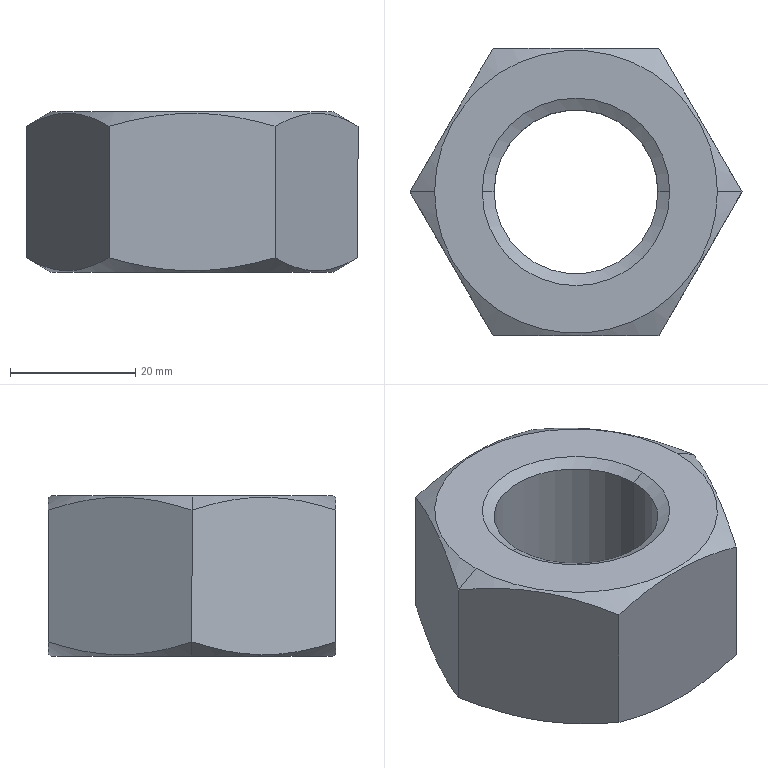Part | SolidWorks | features RevCut 2, Chamfer 1, Extrusion 1, LPattern 1 | 1 solid | 18 faces | box 53.116 x 46 x 25.6 mm | volume 32625 mm3 | cone 8 | plane 8 | cylinder 2 | commonest cylinder face diameters 26.211 x2
STEP:
#1=CARTESIAN_POINT('',(-13.106,0.,-1.094));
#2=VERTEX_POINT('',#1);
#3=CARTESIAN_POINT('',(13.106,0.,-1.094));
#4=VERTEX_POINT('',#3);
#5=CARTESIAN_POINT('',(0.,0.,-1.094));
#6=DIRECTION('',(0.,0.,1.));
#7=DIRECTION('',(1.,0.,0.));
#8=AXIS2_PLACEMENT_3D('',#5,#6,#7);
#9=CIRCLE('',#8,13.106);
#10=EDGE_CURVE('',#2,#4,#9,.T.);
#11=ORIENTED_EDGE('',*,*,#10,.F.);
#12=CARTESIAN_POINT('',(-15.,0.,0.));
#13=VERTEX_POINT('',#12);
#14=CARTESIAN_POINT('',(-13.106,0.,-1.094));
#15=DIRECTION('',(-0.866,0.,0.5));
#16=VECTOR('',#15,1000.);
#17=LINE('',#14,#16);
#18=EDGE_CURVE('',#2,#13,#17,.T.);
#19=ORIENTED_EDGE('',*,*,#18,.T.);
#20=CARTESIAN_POINT('',(15.,0.,0.));
#21=VERTEX_POINT('',#20);
#22=CARTESIAN_POINT('',(0.,0.,0.));
#23=DIRECTION('',(0.,0.,-1.));
#24=DIRECTION('',(1.,0.,0.));
#25=AXIS2_PLACEMENT_3D('',#22,#23,#24);
#26=CIRCLE('',#25,15.);
#27=EDGE_CURVE('',#21,#13,#26,.T.);
#28=ORIENTED_EDGE('',*,*,#27,.F.);
#29=CARTESIAN_POINT('',(13.106,0.,-1.094));
#30=DIRECTION('',(0.866,0.,0.5));
#31=VECTOR('',#30,1000.);
#32=LINE('',#29,#31);
#33=EDGE_CURVE('',#4,#21,#32,.T.);
#34=ORIENTED_EDGE('',*,*,#33,.F.);
#35=EDGE_LOOP('',(#11,#19,#28,#34));
#36=FACE_OUTER_BOUND('',#35,.T.);
#37=CARTESIAN_POINT('',(0.,0.,-1.094));
#38=DIRECTION('',(0.,0.,1.));
#39=DIRECTION('',(1.,0.,0.));
#40=AXIS2_PLACEMENT_3D('',#37,#38,#39);
#41=CONICAL_SURFACE('',#40,13.106,1.047);
#42=ADVANCED_FACE('',(#36),#41,.F.);
#43=CARTESIAN_POINT('',(13.106,0.,-23.705));
#44=VERTEX_POINT('',#43);
#45=CARTESIAN_POINT('',(-13.106,0.,-23.705));
#46=VERTEX_POINT('',#45);
#47=CARTESIAN_POINT('',(0.,0.,-23.705));
#48=DIRECTION('',(0.,0.,-1.));
#49=DIRECTION('',(1.,0.,0.));
#50=AXIS2_PLACEMENT_3D('',#47,#48,#49);
#51=CIRCLE('',#50,13.106);
#52=EDGE_CURVE('',#44,#46,#51,.T.);
#53=ORIENTED_EDGE('',*,*,#52,.F.);
#54=CARTESIAN_POINT('',(14.199,0.,-25.6));
#55=VERTEX_POINT('',#54);
#56=CARTESIAN_POINT('',(14.199,0.,-25.6));
#57=DIRECTION('',(0.5,0.,-0.866));
#58=VECTOR('',#57,1000.);
#59=LINE('',#56,#58);
#60=EDGE_CURVE('',#44,#55,#59,.T.);
#61=ORIENTED_EDGE('',*,*,#60,.T.);
#62=CARTESIAN_POINT('',(-14.199,0.,-25.6));
#63=VERTEX_POINT('',#62);
#64=CARTESIAN_POINT('',(0.,0.,-25.6));
#65=DIRECTION('',(0.,0.,1.));
#66=DIRECTION('',(1.,0.,0.));
#67=AXIS2_PLACEMENT_3D('',#64,#65,#66);
#68=CIRCLE('',#67,14.199);
#69=EDGE_CURVE('',#63,#55,#68,.T.);
#70=ORIENTED_EDGE('',*,*,#69,.F.);
#71=CARTESIAN_POINT('',(-14.199,0.,-25.6));
#72=DIRECTION('',(-0.5,0.,-0.866));
#73=VECTOR('',#72,1000.);
#74=LINE('',#71,#73);
#75=EDGE_CURVE('',#46,#63,#74,.T.);
#76=ORIENTED_EDGE('',*,*,#75,.F.);
#77=EDGE_LOOP('',(#53,#61,#70,#76));
#78=FACE_OUTER_BOUND('',#77,.T.);
#79=CARTESIAN_POINT('',(0.,0.,-25.6));
#80=DIRECTION('',(0.,0.,-1.));
#81=DIRECTION('',(-1.,0.,0.));
#82=AXIS2_PLACEMENT_3D('',#79,#80,#81);
#83=CONICAL_SURFACE('',#82,14.199,0.5236);
#84=ADVANCED_FACE('',(#78),#83,.F.);
#85=CARTESIAN_POINT('',(-22.625,0.,0.));
#86=VERTEX_POINT('',#85);
#87=CARTESIAN_POINT('',(22.625,0.,0.));
#88=VERTEX_POINT('',#87);
#89=CARTESIAN_POINT('',(0.,0.,0.));
#90=DIRECTION('',(0.,0.,-1.));
#91=DIRECTION('',(-1.,0.,0.));
#92=AXIS2_PLACEMENT_3D('',#89,#90,#91);
#93=CIRCLE('',#92,22.625);
#94=EDGE_CURVE('',#86,#88,#93,.T.);
#95=ORIENTED_EDGE('',*,*,#94,.T.);
#96=CARTESIAN_POINT('',(26.558,0.,-2.271));
#97=VERTEX_POINT('',#96);
#98=CARTESIAN_POINT('',(22.625,0.,0.));
#99=DIRECTION('',(0.866,0.,-0.5));
#100=VECTOR('',#99,1000.);
#101=LINE('',#98,#100);
#102=EDGE_CURVE('',#88,#97,#101,.T.);
#103=ORIENTED_EDGE('',*,*,#102,.T.);
#104=CARTESIAN_POINT('',(13.279,23.,-2.271));
#105=VERTEX_POINT('',#104);
#106=CARTESIAN_POINT('',(26.558,0.,-2.271));
#107=CARTESIAN_POINT('',(25.474,1.878,-1.645));
#108=CARTESIAN_POINT('',(24.382,3.769,-1.129));
#109=CARTESIAN_POINT('',(22.175,7.591,-0.4144));
#110=CARTESIAN_POINT('',(21.06,9.523,-0.218));
#111=CARTESIAN_POINT('',(19.649,11.967,-0.2162));
#112=CARTESIAN_POINT('',(19.365,12.458,-0.2279));
#113=CARTESIAN_POINT('',(18.801,13.436,-0.2751));
#114=CARTESIAN_POINT('',(18.519,13.924,-0.3106));
#115=CARTESIAN_POINT('',(17.678,15.381,-0.4511));
#116=CARTESIAN_POINT('',(17.121,16.346,-0.5901));
#117=CARTESIAN_POINT('',(15.459,19.224,-1.127));
#118=CARTESIAN_POINT('',(14.365,21.12,-1.644));
#119=CARTESIAN_POINT('',(13.279,23.,-2.271));
#120=B_SPLINE_CURVE_WITH_KNOTS('',3,(#106,#107,#108,#109,#110,#111,#112,#113,#114,#115,#116,#117,#118,#119),.UNSPECIFIED.,.F.,.F.,(4,2,2,2,2,2,4),(0.000000238,0.006706,0.01341,0.01509,0.01676,0.02012,0.02682),.UNSPECIFIED.);
#121=EDGE_CURVE('',#97,#105,#120,.T.);
#122=ORIENTED_EDGE('',*,*,#121,.T.);
#123=CARTESIAN_POINT('',(-13.279,23.,-2.271));
#124=VERTEX_POINT('',#123);
#125=CARTESIAN_POINT('',(13.279,23.,-2.271));
#126=CARTESIAN_POINT('',(11.133,23.,-1.651));
#127=CARTESIAN_POINT('',(8.958,23.,-1.135));
#128=CARTESIAN_POINT('',(5.632,23.,-0.595));
#129=CARTESIAN_POINT('',(4.511,23.,-0.4541));
#130=CARTESIAN_POINT('',(2.252,23.,-0.2644));
#131=CARTESIAN_POINT('',(1.126,23.,-0.2166));
#132=CARTESIAN_POINT('',(-2.241,23.,-0.2163));
#133=CARTESIAN_POINT('',(-4.471,23.,-0.409));
#134=CARTESIAN_POINT('',(-7.797,23.,-0.9453));
#135=CARTESIAN_POINT('',(-8.904,23.,-1.165));
#136=CARTESIAN_POINT('',(-11.109,23.,-1.673));
#137=CARTESIAN_POINT('',(-12.199,23.,-1.959));
#138=CARTESIAN_POINT('',(-13.279,23.,-2.271));
#139=B_SPLINE_CURVE_WITH_KNOTS('',3,(#125,#126,#127,#128,#129,#130,#131,#132,#133,#134,#135,#136,#137,#138),.UNSPECIFIED.,.F.,.F.,(4,2,2,2,2,2,4),(0.00977,0.01647,0.01982,0.02317,0.02987,0.03323,0.03658),.UNSPECIFIED.);
#140=EDGE_CURVE('',#105,#124,#139,.T.);
#141=ORIENTED_EDGE('',*,*,#140,.T.);
#142=CARTESIAN_POINT('',(-26.558,0.,-2.271));
#143=VERTEX_POINT('',#142);
#144=CARTESIAN_POINT('',(-13.279,23.,-2.271));
#145=CARTESIAN_POINT('',(-14.363,21.122,-1.645));
#146=CARTESIAN_POINT('',(-15.455,19.231,-1.129));
#147=CARTESIAN_POINT('',(-17.662,15.409,-0.4144));
#148=CARTESIAN_POINT('',(-18.777,13.477,-0.218));
#149=CARTESIAN_POINT('',(-20.188,11.033,-0.2162));
#150=CARTESIAN_POINT('',(-20.472,10.542,-0.2279));
#151=CARTESIAN_POINT('',(-21.037,9.564,-0.2751));
#152=CARTESIAN_POINT('',(-21.318,9.076,-0.3106));
#153=CARTESIAN_POINT('',(-22.159,7.619,-0.4511));
#154=CARTESIAN_POINT('',(-22.717,6.654,-0.5901));
#155=CARTESIAN_POINT('',(-24.378,3.776,-1.127));
#156=CARTESIAN_POINT('',(-25.473,1.88,-1.644));
#157=CARTESIAN_POINT('',(-26.558,0.,-2.271));
#158=B_SPLINE_CURVE_WITH_KNOTS('',3,(#144,#145,#146,#147,#148,#149,#150,#151,#152,#153,#154,#155,#156,#157),.UNSPECIFIED.,.F.,.F.,(4,2,2,2,2,2,4),(0.000000238,0.006706,0.01341,0.01509,0.01676,0.02012,0.02682),.UNSPECIFIED.);
#159=EDGE_CURVE('',#124,#143,#158,.T.);
#160=ORIENTED_EDGE('',*,*,#159,.T.);
#161=CARTESIAN_POINT('',(-22.625,0.,0.));
#162=DIRECTION('',(-0.866,0.,-0.5));
#163=VECTOR('',#162,1000.);
#164=LINE('',#161,#163);
#165=EDGE_CURVE('',#86,#143,#164,.T.);
#166=ORIENTED_EDGE('',*,*,#165,.F.);
#167=EDGE_LOOP('',(#95,#103,#122,#141,#160,#166));
#168=FACE_OUTER_BOUND('',#167,.T.);
#169=CARTESIAN_POINT('',(0.,0.,0.));
#170=DIRECTION('',(0.,0.,-1.));
#171=DIRECTION('',(-1.,0.,0.));
#172=AXIS2_PLACEMENT_3D('',#169,#170,#171);
#173=CONICAL_SURFACE('',#172,22.625,1.047);
#174=ADVANCED_FACE('',(#168),#173,.T.);
#175=CARTESIAN_POINT('',(-22.625,0.,-25.6));
#176=VERTEX_POINT('',#175);
#177=CARTESIAN_POINT('',(22.625,0.,-25.6));
#178=VERTEX_POINT('',#177);
#179=CARTESIAN_POINT('',(0.,0.,-25.6));
#180=DIRECTION('',(0.,0.,-1.));
#181=DIRECTION('',(-1.,0.,0.));
#182=AXIS2_PLACEMENT_3D('',#179,#180,#181);
#183=CIRCLE('',#182,22.625);
#184=EDGE_CURVE('',#176,#178,#183,.T.);
#185=ORIENTED_EDGE('',*,*,#184,.F.);
#186=CARTESIAN_POINT('',(-26.558,0.,-23.329));
#187=VERTEX_POINT('',#186);
#188=CARTESIAN_POINT('',(-26.558,0.,-23.329));
#189=DIRECTION('',(-0.866,0.,0.5));
#190=VECTOR('',#189,1000.);
#191=LINE('',#188,#190);
#192=EDGE_CURVE('',#176,#187,#191,.T.);
#193=ORIENTED_EDGE('',*,*,#192,.T.);
#194=CARTESIAN_POINT('',(-13.279,23.,-23.329));
#195=VERTEX_POINT('',#194);
#196=CARTESIAN_POINT('',(-26.558,0.,-23.329));
#197=CARTESIAN_POINT('',(-25.474,1.878,-23.955));
#198=CARTESIAN_POINT('',(-24.382,3.769,-24.471));
#199=CARTESIAN_POINT('',(-22.175,7.591,-25.186));
#200=CARTESIAN_POINT('',(-21.06,9.523,-25.382));
#201=CARTESIAN_POINT('',(-19.649,11.967,-25.384));
#202=CARTESIAN_POINT('',(-19.365,12.458,-25.372));
#203=CARTESIAN_POINT('',(-18.801,13.436,-25.325));
#204=CARTESIAN_POINT('',(-18.519,13.924,-25.289));
#205=CARTESIAN_POINT('',(-17.678,15.381,-25.149));
#206=CARTESIAN_POINT('',(-17.121,16.346,-25.01));
#207=CARTESIAN_POINT('',(-15.459,19.224,-24.473));
#208=CARTESIAN_POINT('',(-14.365,21.12,-23.956));
#209=CARTESIAN_POINT('',(-13.279,23.,-23.329));
#210=B_SPLINE_CURVE_WITH_KNOTS('',3,(#196,#197,#198,#199,#200,#201,#202,#203,#204,#205,#206,#207,#208,#209),.UNSPECIFIED.,.F.,.F.,(4,2,2,2,2,2,4),(0.000000238,0.006706,0.01341,0.01509,0.01676,0.02012,0.02682),.UNSPECIFIED.);
#211=EDGE_CURVE('',#187,#195,#210,.T.);
#212=ORIENTED_EDGE('',*,*,#211,.T.);
#213=CARTESIAN_POINT('',(13.279,23.,-23.329));
#214=VERTEX_POINT('',#213);
#215=CARTESIAN_POINT('',(-13.279,23.,-23.329));
#216=CARTESIAN_POINT('',(-12.199,23.,-23.641));
#217=CARTESIAN_POINT('',(-11.109,23.,-23.927));
#218=CARTESIAN_POINT('',(-8.904,23.,-24.435));
#219=CARTESIAN_POINT('',(-7.797,23.,-24.655));
#220=CARTESIAN_POINT('',(-4.471,23.,-25.191));
#221=CARTESIAN_POINT('',(-2.241,23.,-25.384));
#222=CARTESIAN_POINT('',(1.126,23.,-25.383));
#223=CARTESIAN_POINT('',(2.252,23.,-25.336));
#224=CARTESIAN_POINT('',(4.511,23.,-25.146));
#225=CARTESIAN_POINT('',(5.632,23.,-25.005));
#226=CARTESIAN_POINT('',(8.958,23.,-24.465));
#227=CARTESIAN_POINT('',(11.133,23.,-23.949));
#228=CARTESIAN_POINT('',(13.279,23.,-23.329));
#229=B_SPLINE_CURVE_WITH_KNOTS('',3,(#215,#216,#217,#218,#219,#220,#221,#222,#223,#224,#225,#226,#227,#228),.UNSPECIFIED.,.F.,.F.,(4,2,2,2,2,2,4),(0.02366,0.02702,0.03038,0.0371,0.04045,0.04381,0.05053),.UNSPECIFIED.);
#230=EDGE_CURVE('',#195,#214,#229,.T.);
#231=ORIENTED_EDGE('',*,*,#230,.T.);
#232=CARTESIAN_POINT('',(26.558,0.,-23.329));
#233=VERTEX_POINT('',#232);
#234=CARTESIAN_POINT('',(13.279,23.,-23.329));
#235=CARTESIAN_POINT('',(14.363,21.122,-23.955));
#236=CARTESIAN_POINT('',(15.455,19.231,-24.471));
#237=CARTESIAN_POINT('',(17.662,15.409,-25.186));
#238=CARTESIAN_POINT('',(18.777,13.477,-25.382));
#239=CARTESIAN_POINT('',(20.188,11.033,-25.384));
#240=CARTESIAN_POINT('',(20.472,10.542,-25.372));
#241=CARTESIAN_POINT('',(21.037,9.564,-25.325));
#242=CARTESIAN_POINT('',(21.318,9.076,-25.289));
#243=CARTESIAN_POINT('',(22.159,7.619,-25.149));
#244=CARTESIAN_POINT('',(22.717,6.654,-25.01));
#245=CARTESIAN_POINT('',(24.378,3.776,-24.473));
#246=CARTESIAN_POINT('',(25.473,1.88,-23.956));
#247=CARTESIAN_POINT('',(26.558,0.,-23.329));
#248=B_SPLINE_CURVE_WITH_KNOTS('',3,(#234,#235,#236,#237,#238,#239,#240,#241,#242,#243,#244,#245,#246,#247),.UNSPECIFIED.,.F.,.F.,(4,2,2,2,2,2,4),(0.000000238,0.006706,0.01341,0.01509,0.01676,0.02012,0.02682),.UNSPECIFIED.);
#249=EDGE_CURVE('',#214,#233,#248,.T.);
#250=ORIENTED_EDGE('',*,*,#249,.T.);
#251=CARTESIAN_POINT('',(26.558,0.,-23.329));
#252=DIRECTION('',(0.866,0.,0.5));
#253=VECTOR('',#252,1000.);
#254=LINE('',#251,#253);
#255=EDGE_CURVE('',#178,#233,#254,.T.);
#256=ORIENTED_EDGE('',*,*,#255,.F.);
#257=EDGE_LOOP('',(#185,#193,#212,#231,#250,#256));
#258=FACE_OUTER_BOUND('',#257,.T.);
#259=CARTESIAN_POINT('',(0.,0.,-23.329));
#260=DIRECTION('',(0.,0.,1.));
#261=DIRECTION('',(1.,0.,0.));
#262=AXIS2_PLACEMENT_3D('',#259,#260,#261);
#263=CONICAL_SURFACE('',#262,26.558,1.047);
#264=ADVANCED_FACE('',(#258),#263,.T.);
#265=ORIENTED_EDGE('',*,*,#52,.T.);
#266=CARTESIAN_POINT('',(-13.106,0.,-25.6));
#267=DIRECTION('',(0.,0.,1.));
#268=VECTOR('',#267,1000.);
#269=LINE('',#266,#268);
#270=EDGE_CURVE('',#46,#2,#269,.T.);
#271=ORIENTED_EDGE('',*,*,#270,.T.);
#272=ORIENTED_EDGE('',*,*,#10,.T.);
#273=CARTESIAN_POINT('',(13.106,0.,-25.6));
#274=DIRECTION('',(0.,0.,1.));
#275=VECTOR('',#274,1000.);
#276=LINE('',#273,#275);
#277=EDGE_CURVE('',#44,#4,#276,.T.);
#278=ORIENTED_EDGE('',*,*,#277,.F.);
#279=EDGE_LOOP('',(#265,#271,#272,#278));
#280=FACE_OUTER_BOUND('',#279,.T.);
#281=CARTESIAN_POINT('',(0.,0.,-25.6));
#282=DIRECTION('',(0.,0.,1.));
#283=DIRECTION('',(1.,0.,0.));
#284=AXIS2_PLACEMENT_3D('',#281,#282,#283);
#285=CYLINDRICAL_SURFACE('',#284,13.106);
#286=ADVANCED_FACE('',(#280),#285,.F.);
#287=CARTESIAN_POINT('',(13.279,-23.,-2.271));
#288=VERTEX_POINT('',#287);
#289=CARTESIAN_POINT('',(13.279,-23.,-2.271));
#290=CARTESIAN_POINT('',(14.363,-21.122,-1.645));
#291=CARTESIAN_POINT('',(15.455,-19.231,-1.129));
#292=CARTESIAN_POINT('',(17.662,-15.409,-0.4144));
#293=CARTESIAN_POINT('',(18.777,-13.477,-0.218));
#294=CARTESIAN_POINT('',(20.188,-11.033,-0.2162));
#295=CARTESIAN_POINT('',(20.472,-10.542,-0.2279));
#296=CARTESIAN_POINT('',(21.037,-9.564,-0.2751));
#297=CARTESIAN_POINT('',(21.318,-9.076,-0.3106));
#298=CARTESIAN_POINT('',(22.159,-7.619,-0.4511));
#299=CARTESIAN_POINT('',(22.717,-6.654,-0.5901));
#300=CARTESIAN_POINT('',(24.378,-3.776,-1.127));
#301=CARTESIAN_POINT('',(25.473,-1.88,-1.644));
#302=CARTESIAN_POINT('',(26.558,0.,-2.271));
#303=B_SPLINE_CURVE_WITH_KNOTS('',3,(#289,#290,#291,#292,#293,#294,#295,#296,#297,#298,#299,#300,#301,#302),.UNSPECIFIED.,.F.,.F.,(4,2,2,2,2,2,4),(0.000000238,0.006706,0.01341,0.01509,0.01676,0.02012,0.02682),.UNSPECIFIED.);
#304=EDGE_CURVE('',#288,#97,#303,.T.);
#305=ORIENTED_EDGE('',*,*,#304,.F.);
#306=CARTESIAN_POINT('',(13.279,-23.,-23.329));
#307=VERTEX_POINT('',#306);
#308=CARTESIAN_POINT('',(13.279,-23.,-25.6));
#309=DIRECTION('',(0.,0.,1.));
#310=VECTOR('',#309,1000.);
#311=LINE('',#308,#310);
#312=EDGE_CURVE('',#307,#288,#311,.T.);
#313=ORIENTED_EDGE('',*,*,#312,.F.);
#314=CARTESIAN_POINT('',(26.558,0.,-23.329));
#315=CARTESIAN_POINT('',(25.474,-1.878,-23.955));
#316=CARTESIAN_POINT('',(24.382,-3.769,-24.471));
#317=CARTESIAN_POINT('',(22.175,-7.591,-25.186));
#318=CARTESIAN_POINT('',(21.06,-9.523,-25.382));
#319=CARTESIAN_POINT('',(19.649,-11.967,-25.384));
#320=CARTESIAN_POINT('',(19.365,-12.458,-25.372));
#321=CARTESIAN_POINT('',(18.801,-13.436,-25.325));
#322=CARTESIAN_POINT('',(18.519,-13.924,-25.289));
#323=CARTESIAN_POINT('',(17.678,-15.381,-25.149));
#324=CARTESIAN_POINT('',(17.121,-16.346,-25.01));
#325=CARTESIAN_POINT('',(15.459,-19.224,-24.473));
#326=CARTESIAN_POINT('',(14.365,-21.12,-23.956));
#327=CARTESIAN_POINT('',(13.279,-23.,-23.329));
#328=B_SPLINE_CURVE_WITH_KNOTS('',3,(#314,#315,#316,#317,#318,#319,#320,#321,#322,#323,#324,#325,#326,#327),.UNSPECIFIED.,.F.,.F.,(4,2,2,2,2,2,4),(0.000000238,0.006706,0.01341,0.01509,0.01676,0.02012,0.02682),.UNSPECIFIED.);
#329=EDGE_CURVE('',#233,#307,#328,.T.);
#330=ORIENTED_EDGE('',*,*,#329,.F.);
#331=CARTESIAN_POINT('',(26.558,0.,-25.6));
#332=DIRECTION('',(0.,0.,1.));
#333=VECTOR('',#332,1000.);
#334=LINE('',#331,#333);
#335=EDGE_CURVE('',#233,#97,#334,.T.);
#336=ORIENTED_EDGE('',*,*,#335,.T.);
#337=EDGE_LOOP('',(#305,#313,#330,#336));
#338=FACE_OUTER_BOUND('',#337,.T.);
#339=CARTESIAN_POINT('',(13.279,-23.,-25.6));
#340=DIRECTION('',(0.866,-0.5,0.));
#341=DIRECTION('',(0.5,0.866,0.));
#342=AXIS2_PLACEMENT_3D('',#339,#340,#341);
#343=PLANE('',#342);
#344=ADVANCED_FACE('',(#338),#343,.T.);
#345=CARTESIAN_POINT('',(-13.279,-23.,-2.271));
#346=VERTEX_POINT('',#345);
#347=CARTESIAN_POINT('',(-13.279,-23.,-2.271));
#348=CARTESIAN_POINT('',(-12.199,-23.,-1.959));
#349=CARTESIAN_POINT('',(-11.109,-23.,-1.673));
#350=CARTESIAN_POINT('',(-8.904,-23.,-1.165));
#351=CARTESIAN_POINT('',(-7.797,-23.,-0.9453));
#352=CARTESIAN_POINT('',(-4.471,-23.,-0.409));
#353=CARTESIAN_POINT('',(-2.241,-23.,-0.2163));
#354=CARTESIAN_POINT('',(1.126,-23.,-0.2166));
#355=CARTESIAN_POINT('',(2.252,-23.,-0.2644));
#356=CARTESIAN_POINT('',(4.511,-23.,-0.4541));
#357=CARTESIAN_POINT('',(5.632,-23.,-0.595));
#358=CARTESIAN_POINT('',(8.958,-23.,-1.135));
#359=CARTESIAN_POINT('',(11.133,-23.,-1.651));
#360=CARTESIAN_POINT('',(13.279,-23.,-2.271));
#361=B_SPLINE_CURVE_WITH_KNOTS('',3,(#347,#348,#349,#350,#351,#352,#353,#354,#355,#356,#357,#358,#359,#360),.UNSPECIFIED.,.F.,.F.,(4,2,2,2,2,2,4),(0.02366,0.02702,0.03038,0.0371,0.04045,0.04381,0.05053),.UNSPECIFIED.);
#362=EDGE_CURVE('',#346,#288,#361,.T.);
#363=ORIENTED_EDGE('',*,*,#362,.F.);
#364=CARTESIAN_POINT('',(-13.279,-23.,-23.329));
#365=VERTEX_POINT('',#364);
#366=CARTESIAN_POINT('',(-13.279,-23.,-25.6));
#367=DIRECTION('',(0.,0.,1.));
#368=VECTOR('',#367,1000.);
#369=LINE('',#366,#368);
#370=EDGE_CURVE('',#365,#346,#369,.T.);
#371=ORIENTED_EDGE('',*,*,#370,.F.);
#372=CARTESIAN_POINT('',(13.279,-23.,-23.329));
#373=CARTESIAN_POINT('',(11.133,-23.,-23.949));
#374=CARTESIAN_POINT('',(8.958,-23.,-24.465));
#375=CARTESIAN_POINT('',(5.632,-23.,-25.005));
#376=CARTESIAN_POINT('',(4.511,-23.,-25.146));
#377=CARTESIAN_POINT('',(2.252,-23.,-25.336));
#378=CARTESIAN_POINT('',(1.126,-23.,-25.383));
#379=CARTESIAN_POINT('',(-2.241,-23.,-25.384));
#380=CARTESIAN_POINT('',(-4.471,-23.,-25.191));
#381=CARTESIAN_POINT('',(-7.797,-23.,-24.655));
#382=CARTESIAN_POINT('',(-8.904,-23.,-24.435));
#383=CARTESIAN_POINT('',(-11.109,-23.,-23.927));
#384=CARTESIAN_POINT('',(-12.199,-23.,-23.641));
#385=CARTESIAN_POINT('',(-13.279,-23.,-23.329));
#386=B_SPLINE_CURVE_WITH_KNOTS('',3,(#372,#373,#374,#375,#376,#377,#378,#379,#380,#381,#382,#383,#384,#385),.UNSPECIFIED.,.F.,.F.,(4,2,2,2,2,2,4),(0.00977,0.01647,0.01982,0.02317,0.02987,0.03323,0.03658),.UNSPECIFIED.);
#387=EDGE_CURVE('',#307,#365,#386,.T.);
#388=ORIENTED_EDGE('',*,*,#387,.F.);
#389=ORIENTED_EDGE('',*,*,#312,.T.);
#390=EDGE_LOOP('',(#363,#371,#388,#389));
#391=FACE_OUTER_BOUND('',#390,.T.);
#392=CARTESIAN_POINT('',(-13.279,-23.,-25.6));
#393=DIRECTION('',(0.,-1.,0.));
#394=DIRECTION('',(0.,0.,-1.));
#395=AXIS2_PLACEMENT_3D('',#392,#393,#394);
#396=PLANE('',#395);
#397=ADVANCED_FACE('',(#391),#396,.T.);
#398=CARTESIAN_POINT('',(-26.558,0.,-2.271));
#399=CARTESIAN_POINT('',(-25.474,-1.878,-1.645));
#400=CARTESIAN_POINT('',(-24.382,-3.769,-1.129));
#401=CARTESIAN_POINT('',(-22.175,-7.591,-0.4144));
#402=CARTESIAN_POINT('',(-21.06,-9.523,-0.218));
#403=CARTESIAN_POINT('',(-19.649,-11.967,-0.2162));
#404=CARTESIAN_POINT('',(-19.365,-12.458,-0.2279));
#405=CARTESIAN_POINT('',(-18.801,-13.436,-0.2751));
#406=CARTESIAN_POINT('',(-18.519,-13.924,-0.3106));
#407=CARTESIAN_POINT('',(-17.678,-15.381,-0.4511));
#408=CARTESIAN_POINT('',(-17.121,-16.346,-0.5901));
#409=CARTESIAN_POINT('',(-15.459,-19.224,-1.127));
#410=CARTESIAN_POINT('',(-14.365,-21.12,-1.644));
#411=CARTESIAN_POINT('',(-13.279,-23.,-2.271));
#412=B_SPLINE_CURVE_WITH_KNOTS('',3,(#398,#399,#400,#401,#402,#403,#404,#405,#406,#407,#408,#409,#410,#411),.UNSPECIFIED.,.F.,.F.,(4,2,2,2,2,2,4),(0.000000238,0.006706,0.01341,0.01509,0.01676,0.02012,0.02682),.UNSPECIFIED.);
#413=EDGE_CURVE('',#143,#346,#412,.T.);
#414=ORIENTED_EDGE('',*,*,#413,.F.);
#415=CARTESIAN_POINT('',(-26.558,0.,-25.6));
#416=DIRECTION('',(0.,0.,1.));
#417=VECTOR('',#416,1000.);
#418=LINE('',#415,#417);
#419=EDGE_CURVE('',#187,#143,#418,.T.);
#420=ORIENTED_EDGE('',*,*,#419,.F.);
#421=CARTESIAN_POINT('',(-13.279,-23.,-23.329));
#422=CARTESIAN_POINT('',(-14.363,-21.122,-23.955));
#423=CARTESIAN_POINT('',(-15.455,-19.231,-24.471));
#424=CARTESIAN_POINT('',(-17.662,-15.409,-25.186));
#425=CARTESIAN_POINT('',(-18.777,-13.477,-25.382));
#426=CARTESIAN_POINT('',(-20.188,-11.033,-25.384));
#427=CARTESIAN_POINT('',(-20.472,-10.542,-25.372));
#428=CARTESIAN_POINT('',(-21.037,-9.564,-25.325));
#429=CARTESIAN_POINT('',(-21.318,-9.076,-25.289));
#430=CARTESIAN_POINT('',(-22.159,-7.619,-25.149));
#431=CARTESIAN_POINT('',(-22.717,-6.654,-25.01));
#432=CARTESIAN_POINT('',(-24.378,-3.776,-24.473));
#433=CARTESIAN_POINT('',(-25.473,-1.88,-23.956));
#434=CARTESIAN_POINT('',(-26.558,0.,-23.329));
#435=B_SPLINE_CURVE_WITH_KNOTS('',3,(#421,#422,#423,#424,#425,#426,#427,#428,#429,#430,#431,#432,#433,#434),.UNSPECIFIED.,.F.,.F.,(4,2,2,2,2,2,4),(0.000000238,0.006706,0.01341,0.01509,0.01676,0.02012,0.02682),.UNSPECIFIED.);
#436=EDGE_CURVE('',#365,#187,#435,.T.);
#437=ORIENTED_EDGE('',*,*,#436,.F.);
#438=ORIENTED_EDGE('',*,*,#370,.T.);
#439=EDGE_LOOP('',(#414,#420,#437,#438));
#440=FACE_OUTER_BOUND('',#439,.T.);
#441=CARTESIAN_POINT('',(-26.558,0.,-25.6));
#442=DIRECTION('',(-0.866,-0.5,0.));
#443=DIRECTION('',(0.5,-0.866,0.));
#444=AXIS2_PLACEMENT_3D('',#441,#442,#443);
#445=PLANE('',#444);
#446=ADVANCED_FACE('',(#440),#445,.T.);
#447=ORIENTED_EDGE('',*,*,#159,.F.);
#448=CARTESIAN_POINT('',(-13.279,23.,-25.6));
#449=DIRECTION('',(0.,0.,1.));
#450=VECTOR('',#449,1000.);
#451=LINE('',#448,#450);
#452=EDGE_CURVE('',#195,#124,#451,.T.);
#453=ORIENTED_EDGE('',*,*,#452,.F.);
#454=ORIENTED_EDGE('',*,*,#211,.F.);
#455=ORIENTED_EDGE('',*,*,#419,.T.);
#456=EDGE_LOOP('',(#447,#453,#454,#455));
#457=FACE_OUTER_BOUND('',#456,.T.);
#458=CARTESIAN_POINT('',(-13.279,23.,-25.6));
#459=DIRECTION('',(-0.866,0.5,0.));
#460=DIRECTION('',(-0.5,-0.866,0.));
#461=AXIS2_PLACEMENT_3D('',#458,#459,#460);
#462=PLANE('',#461);
#463=ADVANCED_FACE('',(#457),#462,.T.);
#464=ORIENTED_EDGE('',*,*,#140,.F.);
#465=CARTESIAN_POINT('',(13.279,23.,-25.6));
#466=DIRECTION('',(0.,0.,1.));
#467=VECTOR('',#466,1000.);
#468=LINE('',#465,#467);
#469=EDGE_CURVE('',#214,#105,#468,.T.);
#470=ORIENTED_EDGE('',*,*,#469,.F.);
#471=ORIENTED_EDGE('',*,*,#230,.F.);
#472=ORIENTED_EDGE('',*,*,#452,.T.);
#473=EDGE_LOOP('',(#464,#470,#471,#472));
#474=FACE_OUTER_BOUND('',#473,.T.);
#475=CARTESIAN_POINT('',(13.279,23.,-25.6));
#476=DIRECTION('',(0.,1.,0.));
#477=DIRECTION('',(0.,0.,1.));
#478=AXIS2_PLACEMENT_3D('',#475,#476,#477);
#479=PLANE('',#478);
#480=ADVANCED_FACE('',(#474),#479,.T.);
#481=ORIENTED_EDGE('',*,*,#121,.F.);
#482=ORIENTED_EDGE('',*,*,#335,.F.);
#483=ORIENTED_EDGE('',*,*,#249,.F.);
#484=ORIENTED_EDGE('',*,*,#469,.T.);
#485=EDGE_LOOP('',(#481,#482,#483,#484));
#486=FACE_OUTER_BOUND('',#485,.T.);
#487=CARTESIAN_POINT('',(26.558,0.,-25.6));
#488=DIRECTION('',(0.866,0.5,0.));
#489=DIRECTION('',(-0.5,0.866,0.));
#490=AXIS2_PLACEMENT_3D('',#487,#488,#489);
#491=PLANE('',#490);
#492=ADVANCED_FACE('',(#486),#491,.T.);
#493=ORIENTED_EDGE('',*,*,#69,.T.);
#494=CARTESIAN_POINT('',(0.,0.,-25.6));
#495=DIRECTION('',(0.,0.,1.));
#496=DIRECTION('',(1.,0.,0.));
#497=AXIS2_PLACEMENT_3D('',#494,#495,#496);
#498=CIRCLE('',#497,14.199);
#499=EDGE_CURVE('',#55,#63,#498,.T.);
#500=ORIENTED_EDGE('',*,*,#499,.T.);
#501=EDGE_LOOP('',(#493,#500));
#502=FACE_BOUND('',#501,.T.);
#503=CARTESIAN_POINT('',(0.,0.,-25.6));
#504=DIRECTION('',(0.,0.,-1.));
#505=DIRECTION('',(-1.,0.,0.));
#506=AXIS2_PLACEMENT_3D('',#503,#504,#505);
#507=CIRCLE('',#506,22.625);
#508=EDGE_CURVE('',#178,#176,#507,.T.);
#509=ORIENTED_EDGE('',*,*,#508,.T.);
#510=ORIENTED_EDGE('',*,*,#184,.T.);
#511=EDGE_LOOP('',(#509,#510));
#512=FACE_OUTER_BOUND('',#511,.T.);
#513=CARTESIAN_POINT('',(26.558,0.,-25.6));
#514=DIRECTION('',(0.,0.,1.));
#515=DIRECTION('',(1.,0.,0.));
#516=AXIS2_PLACEMENT_3D('',#513,#514,#515);
#517=PLANE('',#516);
#518=ADVANCED_FACE('',(#502,#512),#517,.F.);
#519=ORIENTED_EDGE('',*,*,#27,.T.);
#520=CARTESIAN_POINT('',(0.,0.,0.));
#521=DIRECTION('',(0.,0.,-1.));
#522=DIRECTION('',(1.,0.,0.));
#523=AXIS2_PLACEMENT_3D('',#520,#521,#522);
#524=CIRCLE('',#523,15.);
#525=EDGE_CURVE('',#13,#21,#524,.T.);
#526=ORIENTED_EDGE('',*,*,#525,.T.);
#527=EDGE_LOOP('',(#519,#526));
#528=FACE_BOUND('',#527,.T.);
#529=ORIENTED_EDGE('',*,*,#94,.F.);
#530=CARTESIAN_POINT('',(0.,0.,0.));
#531=DIRECTION('',(0.,0.,-1.));
#532=DIRECTION('',(-1.,0.,0.));
#533=AXIS2_PLACEMENT_3D('',#530,#531,#532);
#534=CIRCLE('',#533,22.625);
#535=EDGE_CURVE('',#88,#86,#534,.T.);
#536=ORIENTED_EDGE('',*,*,#535,.F.);
#537=EDGE_LOOP('',(#529,#536));
#538=FACE_OUTER_BOUND('',#537,.T.);
#539=CARTESIAN_POINT('',(26.558,0.,0.));
#540=DIRECTION('',(0.,0.,1.));
#541=DIRECTION('',(1.,0.,0.));
#542=AXIS2_PLACEMENT_3D('',#539,#540,#541);
#543=PLANE('',#542);
#544=ADVANCED_FACE('',(#528,#538),#543,.T.);
#545=ORIENTED_EDGE('',*,*,#270,.F.);
#546=CARTESIAN_POINT('',(0.,0.,-23.705));
#547=DIRECTION('',(0.,0.,-1.));
#548=DIRECTION('',(1.,0.,0.));
#549=AXIS2_PLACEMENT_3D('',#546,#547,#548);
#550=CIRCLE('',#549,13.106);
#551=EDGE_CURVE('',#46,#44,#550,.T.);
#552=ORIENTED_EDGE('',*,*,#551,.T.);
#553=ORIENTED_EDGE('',*,*,#277,.T.);
#554=CARTESIAN_POINT('',(0.,0.,-1.094));
#555=DIRECTION('',(0.,0.,1.));
#556=DIRECTION('',(1.,0.,0.));
#557=AXIS2_PLACEMENT_3D('',#554,#555,#556);
#558=CIRCLE('',#557,13.106);
#559=EDGE_CURVE('',#4,#2,#558,.T.);
#560=ORIENTED_EDGE('',*,*,#559,.T.);
#561=EDGE_LOOP('',(#545,#552,#553,#560));
#562=FACE_OUTER_BOUND('',#561,.T.);
#563=CARTESIAN_POINT('',(0.,0.,-25.6));
#564=DIRECTION('',(0.,0.,1.));
#565=DIRECTION('',(1.,0.,0.));
#566=AXIS2_PLACEMENT_3D('',#563,#564,#565);
#567=CYLINDRICAL_SURFACE('',#566,13.106);
#568=ADVANCED_FACE('',(#562),#567,.F.);
#569=ORIENTED_EDGE('',*,*,#192,.F.);
#570=ORIENTED_EDGE('',*,*,#508,.F.);
#571=ORIENTED_EDGE('',*,*,#255,.T.);
#572=ORIENTED_EDGE('',*,*,#329,.T.);
#573=ORIENTED_EDGE('',*,*,#387,.T.);
#574=ORIENTED_EDGE('',*,*,#436,.T.);
#575=EDGE_LOOP('',(#569,#570,#571,#572,#573,#574));
#576=FACE_OUTER_BOUND('',#575,.T.);
#577=CARTESIAN_POINT('',(0.,0.,-23.329));
#578=DIRECTION('',(0.,0.,1.));
#579=DIRECTION('',(1.,0.,0.));
#580=AXIS2_PLACEMENT_3D('',#577,#578,#579);
#581=CONICAL_SURFACE('',#580,26.558,1.047);
#582=ADVANCED_FACE('',(#576),#581,.T.);
#583=ORIENTED_EDGE('',*,*,#102,.F.);
#584=ORIENTED_EDGE('',*,*,#535,.T.);
#585=ORIENTED_EDGE('',*,*,#165,.T.);
#586=ORIENTED_EDGE('',*,*,#413,.T.);
#587=ORIENTED_EDGE('',*,*,#362,.T.);
#588=ORIENTED_EDGE('',*,*,#304,.T.);
#589=EDGE_LOOP('',(#583,#584,#585,#586,#587,#588));
#590=FACE_OUTER_BOUND('',#589,.T.);
#591=CARTESIAN_POINT('',(0.,0.,0.));
#592=DIRECTION('',(0.,0.,-1.));
#593=DIRECTION('',(-1.,0.,0.));
#594=AXIS2_PLACEMENT_3D('',#591,#592,#593);
#595=CONICAL_SURFACE('',#594,22.625,1.047);
#596=ADVANCED_FACE('',(#590),#595,.T.);
#597=ORIENTED_EDGE('',*,*,#60,.F.);
#598=ORIENTED_EDGE('',*,*,#551,.F.);
#599=ORIENTED_EDGE('',*,*,#75,.T.);
#600=ORIENTED_EDGE('',*,*,#499,.F.);
#601=EDGE_LOOP('',(#597,#598,#599,#600));
#602=FACE_OUTER_BOUND('',#601,.T.);
#603=CARTESIAN_POINT('',(0.,0.,-25.6));
#604=DIRECTION('',(0.,0.,-1.));
#605=DIRECTION('',(-1.,0.,0.));
#606=AXIS2_PLACEMENT_3D('',#603,#604,#605);
#607=CONICAL_SURFACE('',#606,14.199,0.5236);
#608=ADVANCED_FACE('',(#602),#607,.F.);
#609=ORIENTED_EDGE('',*,*,#18,.F.);
#610=ORIENTED_EDGE('',*,*,#559,.F.);
#611=ORIENTED_EDGE('',*,*,#33,.T.);
#612=ORIENTED_EDGE('',*,*,#525,.F.);
#613=EDGE_LOOP('',(#609,#610,#611,#612));
#614=FACE_OUTER_BOUND('',#613,.T.);
#615=CARTESIAN_POINT('',(0.,0.,-1.094));
#616=DIRECTION('',(0.,0.,1.));
#617=DIRECTION('',(1.,0.,0.));
#618=AXIS2_PLACEMENT_3D('',#615,#616,#617);
#619=CONICAL_SURFACE('',#618,13.106,1.047);
#620=ADVANCED_FACE('',(#614),#619,.F.);
#621=CLOSED_SHELL('',(#42,#84,#174,#264,#286,#344,#397,#446,#463,#480,#492,#518,#544,#568,#582,#596,#608,#620));
#622=MANIFOLD_SOLID_BREP('',#621);
#623=CARTESIAN_POINT('',(0.,0.,0.));
#624=DIRECTION('',(0.,0.,1.));
#625=DIRECTION('',(1.,0.,0.));
#626=AXIS2_PLACEMENT_3D('',#623,#624,#625);
#627=(LENGTH_UNIT()NAMED_UNIT(*)SI_UNIT(.MILLI.,.METRE.));
#628=UNCERTAINTY_MEASURE_WITH_UNIT(LENGTH_MEASURE(0.00001),#627,'','');
#629=(NAMED_UNIT(*)PLANE_ANGLE_UNIT()SI_UNIT($,.RADIAN.));
#630=(NAMED_UNIT(*)SI_UNIT($,.STERADIAN.)SOLID_ANGLE_UNIT());
#631=(GEOMETRIC_REPRESENTATION_CONTEXT(3)GLOBAL_UNCERTAINTY_ASSIGNED_CONTEXT((#628))GLOBAL_UNIT_ASSIGNED_CONTEXT((#627,#629,#630))REPRESENTATION_CONTEXT('',''));
#632=ADVANCED_BREP_SHAPE_REPRESENTATION('',(#622,#626),#631);